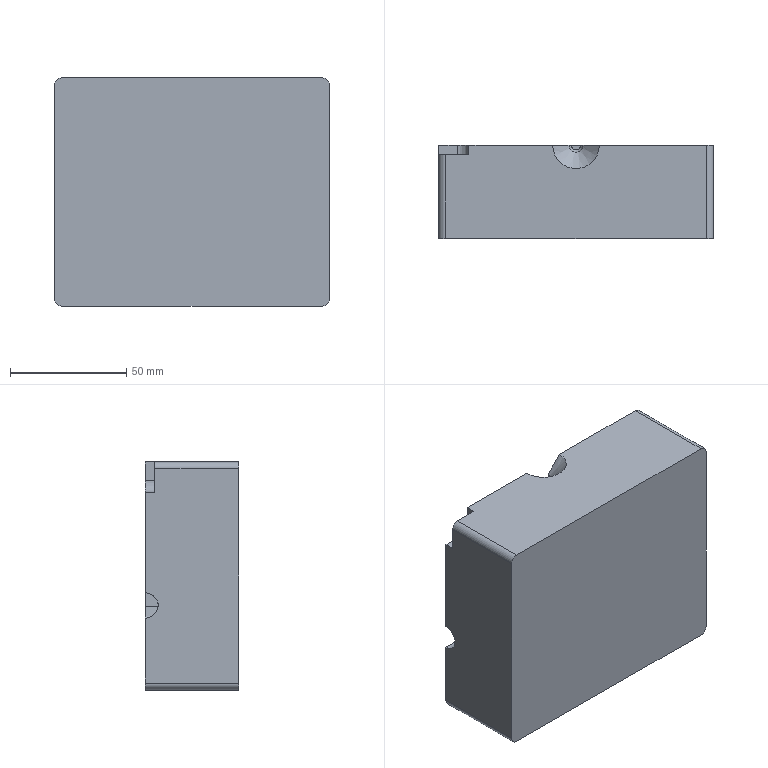NC program | NX | posted with a generic post | part box 118 x 40 x 98 mm
Lines 1488 to 2680 of 39656:
(CAVITY_MILL_COPY , TOOL : D4)
N2974 M6
N2976 G54
N2978 G17 G0 G90 X-30.742 Y-9.957 S0 M3
N2980 G43 Z30. H0
N2982 Z-0.963
N2984 G94 G1 Y-10.759 F250.
N2986 Y-17.85
N2988 X-31.058
N2990 Y-10.759
N2992 G2 X-33.146 Y-9.385 R2.52
N2994 X-33.058 Y-10.049 R2.146
N2996 G1 Y-19.85
N2998 X-28.742
N3000 Y-9.865
N3002 G2 X-28.696 Y-9.549 R1.086
N3004 G1 X-28.636 Y-9.352
N3006 X-28.053 Y-7.435
N3008 G0 X-33.789 Y-7.253 Z-1.925
N3010 G1 X-32.909 Y-9.083
N3012 X-32.861 Y-9.191
N3014 G2 X-32.701 Y-9.99 R2.527
N3016 G1 X-32.709 Y-10.
N3018 Y-19.814
N3020 G3 X-32.365 Y-19.85 R1.654
N3022 G1 X-29.435
N3024 X-29.112 Y-19.819
N3026 X-29.091 Y-19.815
N3028 Y-10.
N3030 X-29.098 Y-9.99
N3032 G2 X-28.879 Y-9.065 R2.165
N3034 G1 X-27.99 Y-7.245
N3036 G0 X-32.698 Y-7.471 Z-2.888
N3038 G1 X-33.034 Y-8.04
N3040 X-32.523 Y-8.656
N3042 X-32.418 Y-8.792
N3044 G2 X-32.042 Y-10. R2.079
N3046 G1 Y-19.671
N3048 G3 X-30.775 Y-19.785 R4.978
N3050 X-29.758 Y-19.671 R4.359
N3052 G1 Y-10.
N3054 G2 X-29.261 Y-8.64 R2.107
N3056 G1 X-28.745 Y-8.029
N3058 X-29.076 Y-7.457
N3060 G0 X-32.324 Y-7.137 Z-3.85
N3062 G1 X-32.463 Y-7.781
N3064 X-31.779 Y-8.197
N3066 G2 X-30.9 Y-9.216 R2.184
N3068 X-30.024 Y-8.196 R2.052
N3070 G1 X-29.333 Y-7.793
N3072 X-29.482 Y-7.134
N3074 G0 Z30.
N3076 X-34.354 Y-3.075
N3078 Z-0.963
N3080 G1 X-35.516 Y-4.812
N3082 G2 X-37.305 Y-5.764 R2.144
N3084 G1 X-37.919
N3086 Y-7.85
N3088 X-35.21
N3090 G2 X-34.483 Y-7.974 R2.146
N3092 G1 X-32.582 Y-8.651
N3094 G0 X-34.128 Y-2.971 Z-1.925
N3096 G1 X-35.263 Y-4.762
N3098 G2 X-37.084 Y-5.764 R2.157
N3100 G1 X-37.768
N3102 Y-7.85
N3104 X-34.875
N3106 G2 X-34.172 Y-7.965 R2.175
N3108 G1 X-32.249 Y-8.616
N3110 G0 X-33.73 Y-2.932 Z-2.888
N3112 G1 X-34.85 Y-4.742
N3114 G2 X-36.371 Y-5.734 R2.136
N3116 X-36.698 Y-5.764 R1.684
N3118 G1 X-37.51
N3120 Y-7.85
N3122 X-34.243
N3124 G2 X-33.618 Y-7.938 R2.232
N3126 G1 X-32.85 Y-8.161
N3128 X-32.462 Y-7.626
N3130 G0 X-33.123 Y-2.743 Z-3.85
N3132 G1 X-34.197 Y-4.658
N3134 G2 X-34.88 Y-5.395 R2.143
N3136 G1 X-35.172 Y-5.552
N3138 G2 X-36.111 Y-5.764 R2.188
N3140 G1 X-37.138
N3142 Y-7.85
N3144 X-33.069
N3146 G2 X-32.597 Y-7.898 R3.124
N3148 G1 X-31.81 Y-8.04
N3150 X-31.485 Y-7.443
N3152 G0 Z30.
N3154 X-58.08 Y13.101
N3156 Z-2.888
N3158 G1 X-57.261
N3160 X-40.113
N3162 G2 X-38.246 Y15.104 R2.52
N3164 G1 X-38.339 Y15.101
N3166 X-59.
N3168 X-61.015
N3170 X-39.295 Y12.219
N3172 X-40.113
N3174 X-57.261
N3176 G2 X-59. Y10.251 R2.52
N3178 G1 Y10.219
N3180 X-38.769
N3182 X-38.382 Y10.222
N3184 X-38.258 Y10.218
N3186 X-36.248 Y10.108
N3188 G0 Z30.
N3190 X-35.121 Y15.559
N3192 Z-3.85
N3194 G1 X-36.861 Y14.574
N3196 G2 X-37.896 Y14.301 R2.099
N3198 G1 X-58.975
N3200 X-59.
N3202 X-61.006 Y14.297
N3204 X-61. Y11.042
N3206 X-59. Y11.019
N3208 X-58.99
N3210 X-37.904
N3212 G2 X-36.839 Y10.731 R2.116
N3214 G1 X-35.105 Y9.72
N3216 G0 X-34.351 Y15.355 Z-4.814
N3218 G1 X-35.564 Y13.719
N3220 G2 X-37.25 Y12.869 R2.102
N3222 G1 X-37.57 Y12.871
N3224 X-58.975
N3226 X-59.
N3228 X-61.265 Y12.886
N3230 X-61.261 Y12.459
N3232 X-59. Y12.449
N3234 X-58.99
N3236 X-37.236
N3238 G2 X-35.971 Y12.02 R2.076
N3240 X-35.552 Y11.576 R2.175
N3242 G1 X-34.351 Y9.883
N3244 G0 Z30.
N3246 X-35.931 Y6.35
N3248 Z-0.963
N3250 G1 X-36.731
N3252 Y5.55
N3254 Y4.444
N3256 G2 X-36.041 Y4.113 R2.145
N3258 G1 X-34.406 Y2.929
N3260 G0 X-35.752 Y6.401 Z-1.925
N3262 G1 X-36.552
N3264 Y5.601
N3266 Y4.456
N3268 G2 X-35.793 Y4.096 R2.148
N3270 G1 X-34.173 Y2.89
N3272 G0 X-35.443 Y6.455 Z-2.888
N3274 G1 X-36.243
N3276 Y5.655
N3278 Y4.474
N3280 G2 X-35.504 Y4.17 R2.144
N3282 G1 X-33.813 Y3.068
N3284 G0 X-34.988 Y6.572 Z-3.85
N3286 G1 X-35.788
N3288 Y5.772
N3290 Y4.506
N3292 G2 X-34.943 Y4.188 R2.395
N3294 G1 X-33.225 Y3.136
N3296 G0 Z30.
N3298 X-34.351 Y6.757
N3300 Z-4.814
N3302 G1 X-35.151
N3304 Y5.957
N3306 Y4.564
N3308 G3 X-34.772 Y4.475 R4.427
N3310 G2 X-34.184 Y4.273 R2.191
N3312 G1 X-32.371 Y3.347
N3314 G0 Z30.
N3316 X-33.472 Y7.081
N3318 Z-5.778
N3320 G1 X-34.272
N3322 Y6.281
N3324 Y4.663
N3326 G3 X-33.573 Y4.51 R2.774
N3328 G2 X-32.997 Y4.395 R2.36
N3330 G1 X-32.237 Y4.143
N3332 X-31.834 Y4.675
N3334 G0 Z30.
N3336 X-27.389 Y2.955
N3338 Z-0.963
N3340 G1 X-25.745 Y4.124
N3342 G2 X-25.069 Y4.445 R2.143
N3344 G1 Y5.546
N3346 Y6.346
N3348 X-25.869
N3350 G0 X-27.61 Y2.981 Z-1.925
N3352 G1 X-25.953 Y4.135
N3354 G2 X-25.248 Y4.455 R2.149
N3356 G1 Y5.586
N3358 Y6.386
N3360 X-26.048
N3362 G0 X-27.99 Y3.049 Z-2.888
N3364 G1 X-26.303 Y4.163
N3366 G2 X-25.557 Y4.474 R2.153
N3368 G1 Y5.655
N3370 Y6.455
N3372 X-26.357
N3374 G0 X-28.58 Y3.121 Z-3.85
N3376 G1 X-26.843 Y4.198
N3378 G2 X-26.012 Y4.506 R2.239
N3380 G1 Y5.769
N3382 Y6.569
N3384 X-26.812
N3386 G0 X-29.417 Y3.37 Z-4.814
N3388 G1 X-27.611 Y4.277
N3390 G2 X-27.178 Y4.439 R2.146
N3392 G3 X-26.649 Y4.565 R3.444
N3394 G1 Y5.957
N3396 Y6.757
N3398 X-27.449
N3400 G0 Z30.
N3402 X-29.987 Y4.661
N3404 Z-5.778
N3406 G1 X-29.58 Y4.131
N3408 X-28.821 Y4.385
N3410 G2 X-28.295 Y4.497 R2.367
N3412 G3 X-27.528 Y4.663 R3.33
N3414 G1 Y6.281
N3416 Y7.081
N3418 X-28.328
N3420 G0 Z30.
N3422 X-22.377 Y13.101
N3424 Z-2.888
N3426 G1 X-21.092
N3428 X-19.388
N3430 G3 X-18.519 Y13.892 R2.
N3432 G2 X-16.717 Y15.101 R2.52
N3434 G1 X-23.426
N3436 X-23.549 Y15.105
N3438 X-25.552 Y15.217
N3440 G0 Z30.
N3442 X-18.179 Y12.219
N3444 Z-2.888
N3446 G1 X-19.541 Y12.22
N3448 X-20.998
N3450 G3 X-21.991 Y11.376 R2.
N3452 G2 X-23.535 Y10.219 R2.52
N3454 G1 X-23.417 Y10.222
N3456 X-23.181 Y10.219
N3458 X-17.313
N3460 G2 X-17.113 Y10.206 R2.13
N3462 G1 X-15.113 Y9.987
N3464 G0 Z30.
N3466 X-26.692 Y9.728
N3468 Z-3.85
N3470 G1 X-24.953 Y10.736
N3472 G2 X-24.083 Y11.014 R2.125
N3474 G1 X-23.913 Y11.021
N3476 X-23.581 Y11.019
N3478 X-17.287
N3480 G2 X-16.177 Y10.687 R2.053
N3482 G1 X-14.475 Y9.582
N3484 X-14.034 Y15.389
N3486 X-15.89 Y14.5
N3488 X-15.987 Y14.456
N3490 G2 X-16.798 Y14.301 R2.052
N3492 G1 X-23.581
N3494 X-23.892 Y14.297
N3496 G2 X-24.951 Y14.583 R2.119
N3498 G1 X-26.688 Y15.59
N3500 G0 X-27.449 Y9.952 Z-4.814
N3502 G1 X-26.24 Y11.594
N3504 G2 X-24.549 Y12.449 R2.1
N3506 G1 X-17.251
N3508 G2 X-15.587 Y11.58 R2.033
N3510 G1 X-15.522 Y11.481
N3512 X-14.351 Y9.618
N3514 X-13.97 Y15.475
N3516 X-15.424 Y13.642
N3518 G2 X-17.061 Y12.871 R2.039
N3520 G1 X-24.548
N3522 G2 X-26.242 Y13.729 R2.101
N3524 G1 X-27.449 Y15.375
N3526 G0 Z30.
N3528 X-15.428 Y-3.812
N3530 Z-0.963
N3532 G1 X-16.062 Y-3.445
N3534 X-16.573 Y-4.06
N3536 G2 X-20.207 Y-5.764 R4.725
N3538 G1 X-24.495
N3540 G2 X-26.289 Y-4.806 R2.143
N3542 G1 X-27.446 Y-3.062
N3544 X-29.223 Y-8.661
N3546 X-27.324 Y-7.977
N3548 G2 X-26.59 Y-7.85 R2.147
N3550 G1 X-14.726
N3552 X-13.926
N3554 Y-7.05
N3556 G0 X-15.428 Y-3.812 Z-1.925
N3558 G1 X-16.062 Y-3.445
N3560 X-16.573 Y-4.06
N3562 G2 X-20.207 Y-5.764 R4.725
N3564 G1 X-24.716
N3566 G2 X-26.528 Y-4.777 R2.157
N3568 G1 X-27.672 Y-3.004
N3570 X-29.536 Y-8.595
N3572 X-27.612 Y-7.959
N3574 G2 X-26.924 Y-7.85 R2.165
N3576 G1 X-14.726
N3578 X-13.926
N3580 Y-7.05
N3582 G0 X-15.428 Y-3.812 Z-2.888
N3584 G1 X-16.062 Y-3.445
N3586 X-16.573 Y-4.06
N3588 G2 X-20.207 Y-5.764 R4.725
N3590 G1 X-25.102
N3592 G2 X-26.952 Y-4.735 R2.154
N3594 G1 X-28.07 Y-2.912
N3596 X-29.351 Y-7.638
N3598 X-28.96 Y-8.17
N3600 X-28.193 Y-7.942
N3602 G2 X-27.557 Y-7.85 R2.228
N3604 G1 X-14.726
N3606 X-13.926
N3608 Y-7.05
N3610 G0 X-15.428 Y-3.812 Z-3.85
N3612 G1 X-16.062 Y-3.445
N3614 X-16.573 Y-4.06
N3616 G2 X-20.207 Y-5.764 R4.725
N3618 G1 X-25.689
N3620 G2 X-27.521 Y-4.795 R2.22
N3622 G1 X-27.594 Y-4.681
N3624 X-28.677 Y-2.845
N3626 X-30.266 Y-7.417
N3628 X-29.958 Y-8.021
N3630 X-29.169 Y-7.887
N3632 G2 X-28.73 Y-7.85 R2.566
N3634 G1 X-14.726
N3636 X-13.926
N3638 Y-7.05
N3640 G0 Z30.
N3642 X-30.794 Y2.521
N3644 Z-4.814
N3646 G1 Y1.72
N3648 Y-3.598
N3650 G3 X-30.138 Y-5.85 R4.087
N3652 G1 X-31.662
N3654 G3 X-31.006 Y-3.584 R4.091
N3656 G1 Y1.72
N3658 G2 X-33.098 Y3.001 R2.52
N3660 X-33.042 Y2.797 R2.191
N3662 G1 X-32.996 Y2.398
N3664 X-33.006 Y2.371
N3666 Y-3.597
N3668 G2 X-33.979 Y-5.395 R2.091
N3670 X-35.232 Y-5.764 R2.311
N3672 G1 X-36.63
N3674 Y-7.85
N3676 X-14.726
N3678 X-13.926
N3680 Y-7.05
N3682 X-15.428 Y-3.812
N3684 X-16.062 Y-3.445
N3686 X-16.573 Y-4.06
N3688 G2 X-20.207 Y-5.764 R4.725
N3690 G1 X-26.566
N3692 G2 X-27.239 Y-5.667 R2.948
N3694 X-27.578 Y-5.525 R1.364
N3696 X-28.794 Y-3.607 R2.087
N3698 G1 Y2.361
N3700 G2 X-28.68 Y3.05 R2.146
N3702 G1 X-28.028 Y4.969
N3704 G0 Z30.
N3706 X-15.428 Y-3.812
N3708 Z-5.778
N3710 G1 X-16.062 Y-3.445
N3712 X-16.573 Y-4.06
N3714 G2 X-20.207 Y-5.764 R4.725
N3716 G1 X-27.973
N3718 G2 X-29.592 Y-5.195 R2.509
N3720 X-30.322 Y-3.597 R2.013
N3722 G1 Y2.358
N3724 G2 X-29.605 Y3.939 R2.104
N3726 G1 X-29.004 Y4.467
N3728 X-29.25 Y5.079
N3730 X-32.538 Y5.078
N3732 X-32.792 Y4.46
N3734 X-32.19 Y3.934
N3736 G2 X-31.872 Y3.597 R2.36
N3738 X-31.478 Y2.35 R2.
N3740 G1 Y-3.628
N3742 G2 X-32.575 Y-5.452 R2.065
N3744 X-33.827 Y-5.764 R2.67
N3746 G1 X-35.963
N3748 Y-7.85
N3750 X-14.726
N3752 X-13.926
N3754 Y-7.05
N3756 G0 Z30.
N3758 X-30.802 Y50.223
N3760 Z-6.742
N3762 G1 Y48.36
N3764 Y6.616
N3766 X-30.998 Y6.617
N3768 Y48.36
N3770 G2 X-32.581 Y49. R2.52
N3772 G1 X-32.998
N3774 Y4.849
N3776 G3 X-32.374 Y4.705 R3.357
N3778 X-29.576 Y4.686 R12.401
N3780 X-28.802 Y4.848 R4.237
N3782 G1 Y49.
N3784 Y51.004
N3786 G0 Z30.
N3788 X-15.428 Y-3.812
N3790 Z-6.742
N3792 G1 X-16.062 Y-3.445
N3794 X-16.573 Y-4.06
N3796 G2 X-20.207 Y-5.764 R4.725
N3798 G1 X-35.086
N3800 Y-7.85
N3802 X-14.726
N3804 X-13.926
N3806 Y-7.05
N3808 G0 X-15.428 Y-3.812 Z-7.707
N3810 G1 X-16.062 Y-3.445
N3812 X-16.573 Y-4.06
N3814 G2 X-20.207 Y-5.764 R4.725
N3816 G1 X-33.596
N3818 X-33.894 Y-5.776
N3820 Y-7.85
N3822 X-14.726
N3824 X-13.926
N3826 Y-7.05
N3828 G0 X-15.422 Y-3.828 Z-8.671
N3830 G1 X-16.054 Y-3.458
N3832 X-16.568 Y-4.071
N3834 G2 X-19.94 Y-5.756 R4.731
N3836 X-20.207 Y-5.764 R4.725
N3838 G1 X-27.744
N3840 G3 X-30.975 Y-5.844 R72.062
N3842 X-32.076 Y-5.927 R18.052
N3844 G1 Y-7.832
N3846 X-31.974 Y-7.836
N3848 X-31.069 Y-7.85
N3850 X-14.714
N3852 X-13.914
N3854 Y-7.05
N3856 G0 X-14.831 Y-3.815 Z-9.635
N3858 G1 X-15.469 Y-3.48
N3860 X-15.973 Y-4.101
N3862 G2 X-17.236 Y-5.126 R3.966
N3864 X-19.883 Y-5.779 R5.896
N3866 G3 X-25.06 Y-5.994 R79.105
N3868 X-26.853 Y-6.206 R23.699
N3870 G1 Y-7.67
N3872 G3 X-24.38 Y-7.821 R33.331
N3874 G1 X-22.782 Y-7.849
N3876 X-22.62 Y-7.85
N3878 X-14.102
N3880 X-13.302
N3882 Y-7.05
N3884 G0 X-12.915 Y-2.639 Z-10.356
N3886 G1 X-14.194 Y-4.337
N3888 G2 X-14.486 Y-4.657 R2.325
N3890 X-17.42 Y-5.994 R5.27
N3892 G1 X-19.984 Y-6.253
N3894 X-20.157 Y-6.28
N3896 Y-7.613
N3898 G3 X-17.186 Y-7.789 R43.351
N3900 G1 X-16.387 Y-7.811
N3902 X-13.042 Y-7.85
N3904 X-12.204
N3906 X-11.404
N3908 Y-7.05
N3910 G0 Z30.
N3912 X-2.778 Y-8.134
N3914 Z-6.742
N3916 G1 X-2.373 Y-10.493
N3918 G2 X-2.385 Y-11.637 R3.183
N3920 G1 X-2.394 Y-11.678
N3922 X-2.546 Y-12.464
N3924 X-1.761 Y-12.616
N3926 G0 X-2.801 Y-8.096 Z-7.707
N3928 G1 X-2.364 Y-10.45
N3930 G2 X-2.368 Y-11.637 R3.183
N3932 G1 X-2.394 Y-11.767
N3934 X-2.546 Y-12.552
N3936 X-1.761 Y-12.705
N3938 G0 X-2.823 Y-8.052 Z-8.671
N3940 G1 X-2.35 Y-10.398
N3942 G2 X-2.346 Y-11.635 R3.178
N3944 G1 X-2.394 Y-11.881
N3946 X-2.546 Y-12.666
N3948 X-1.761 Y-12.818
N3950 G0 Z30.
N3952 X-0.177 Y-16.227
N3954 Z-9.635
N3956 G1 X-0.02 Y-15.418
N3958 X0. Y-15.318
N3960 X0.02 Y-15.418
N3962 G2 X2.394 Y-17.15 R2.52
N3964 G1 X1.313 Y-11.589
N3966 X1.244 Y-11.418
N3968 G2 X1.7 Y-9.701 R2.141
N3970 G1 X2.207 Y-9.082
N3972 X1.71 Y-8.538
N3974 X-1.733 Y-8.515
N3976 X-2.209 Y-9.052
N3978 X-1.706 Y-9.674
N3980 G2 X-1.23 Y-11.411 R2.247
N3982 G1 X-1.28 Y-11.423
N3984 X-2.394 Y-17.15
N3986 X-2.546 Y-17.936
N3988 X-1.761 Y-18.088
N3990 G0 Z30.
N3992 X-0.061 Y-7.471
N3994 Z-9.135
N3996 G3 X-0.061 Y-7.471 Z-9.185 I0.061 J0.456
N3998 X-0.061 Y-7.471 Z-9.236 I0.061 J0.456
N4000 X-0.061 Y-7.471 Z-9.286 I0.061 J0.456
N4002 X-0.061 Y-7.471 Z-9.337 I0.061 J0.456
N4004 X-0.061 Y-7.471 Z-9.387 I0.061 J0.456
N4006 X-0.061 Y-7.471 Z-9.438 I0.061 J0.456
N4008 X-0.061 Y-7.471 Z-9.488 I0.061 J0.456
N4010 X-0.061 Y-7.471 Z-9.539 I0.061 J0.456
N4012 X-0.061 Y-7.471 Z-9.589 I0.061 J0.456
N4014 X-0.061 Y-7.471 Z-9.639 I0.061 J0.456
N4016 X-0.061 Y-7.471 Z-9.69 I0.061 J0.456
N4018 X-0.061 Y-7.471 Z-9.74 I0.061 J0.456
N4020 X-0.061 Y-7.471 Z-9.791 I0.061 J0.456
N4022 X-0.061 Y-7.471 Z-9.841 I0.061 J0.456
N4024 X-0.061 Y-7.471 Z-9.892 I0.061 J0.456
N4026 X-0.061 Y-7.471 Z-9.942 I0.061 J0.456
N4028 X-0.061 Y-7.471 Z-9.993 I0.061 J0.456
N4030 X-0.061 Y-7.471 Z-10.043 I0.061 J0.456
N4032 X-0.061 Y-7.471 Z-10.094 I0.061 J0.456
N4034 X-0.061 Y-7.471 Z-10.144 I0.061 J0.456
N4036 X-0.061 Y-7.471 Z-10.194 I0.061 J0.456
N4038 X-0.061 Y-7.471 Z-10.245 I0.061 J0.456
N4040 X-0.061 Y-7.471 Z-10.295 I0.061 J0.456
N4042 X-0.061 Y-7.471 Z-10.346 I0.061 J0.456
N4044 X-0.061 Y-7.471 Z-10.396 I0.061 J0.456
N4046 X-0.061 Y-7.471 Z-10.447 I0.061 J0.456
N4048 X-0.061 Y-7.471 Z-10.497 I0.061 J0.456
N4050 X-0.061 Y-7.471 Z-10.548 I0.061 J0.456
N4052 X-0.061 Y-7.471 Z-10.598 I0.061 J0.456
N4054 X-0.061 Y-7.471 Z-10.648 I0.061 J0.456
N4056 X-0.061 Y-7.471 Z-10.699 I0.061 J0.456
N4058 X-0.061 Y-7.471 Z-10.749 I0.061 J0.456
N4060 X-0.061 Y-7.471 Z-10.8 I0.061 J0.456
N4062 X-0.061 Y-7.471 Z-10.85 I0.061 J0.456
N4064 X-0.061 Y-7.471 Z-10.901 I0.061 J0.456
N4066 X-0.061 Y-7.471 Z-10.951 I0.061 J0.456
N4068 X-0.061 Y-7.471 Z-11.002 I0.061 J0.456
N4070 X-0.061 Y-7.471 Z-11.052 I0.061 J0.456
N4072 X-0.061 Y-7.471 Z-11.103 I0.061 J0.456
N4074 X-0.061 Y-7.471 Z-11.153 I0.061 J0.456
N4076 X-0.061 Y-7.471 Z-11.203 I0.061 J0.456
N4078 X-0.061 Y-7.471 Z-11.254 I0.061 J0.456
N4080 X-0.061 Y-7.471 Z-11.304 I0.061 J0.456
N4082 X0. Y-7.475 Z-11.305 R0.46
N4084 X4.197 Y-7.406 R128.083
N4086 G1 Y-6.557
N4088 G3 X-4.197 Y-6.556 R87.806
N4090 G1 Y-7.407
N4092 G3 X0. Y-7.475 R128.083
N4094 G1 Y-6.675
N4096 G0 Z30.
N4098 X-3.997 Y-23.59
N4100 Z-0.963
N4102 G1 X-4.782 Y-23.437
N4104 X-4.935 Y-24.222
N4106 X-5.453 Y-26.888
N4108 X-2.737
N4110 X-1.937
N4112 Y-26.088
N4114 G0 X-3.976 Y-23.573 Z-1.925
N4116 G1 X-4.762 Y-23.42
N4118 X-4.914 Y-24.205
N4120 X-5.432 Y-26.871
N4122 X-2.717
N4124 X-1.917
N4126 Y-26.071
N4128 G0 X-3.956 Y-23.556 Z-2.888
N4130 G1 X-4.741 Y-23.403
N4132 X-4.894 Y-24.189
N4134 X-5.412 Y-26.855
N4136 X-2.696
N4138 X-1.896
N4140 Y-26.055
N4142 G0 X-3.936 Y-23.539 Z-3.85
N4144 G1 X-4.721 Y-23.387
N4146 X-4.874 Y-24.172
N4148 X-5.392 Y-26.838
N4150 X-2.676
N4152 X-1.876
N4154 Y-26.038
N4156 G0 X-3.915 Y-23.522 Z-4.814
N4158 G1 X-4.7 Y-23.37
N4160 X-4.853 Y-24.155
N4162 X-5.371 Y-26.821
N4164 X-2.655
N4166 X-1.855
N4168 Y-26.021
N4170 G0 X-3.895 Y-23.505 Z-5.778
N4172 G1 X-4.68 Y-23.353
N4174 X-4.833 Y-24.138
N4176 X-5.351 Y-26.804
N4178 X-2.635
N4180 X-1.835
N4182 Y-26.004
N4184 G0 X-3.874 Y-23.489 Z-6.742
N4186 G1 X-4.66 Y-23.336
N4188 X-4.812 Y-24.121
N4190 X-5.33 Y-26.787
N4192 X-2.615
N4194 X-1.815
N4196 Y-25.987
N4198 G0 X-3.854 Y-23.472 Z-7.707
N4200 G1 X-4.639 Y-23.319
N4202 X-4.792 Y-24.104
N4204 X-5.31 Y-26.77
N4206 X-2.594
N4208 X-1.794
N4210 Y-25.97
N4212 G0 X-3.828 Y-23.45 Z-8.671
N4214 G1 X-4.613 Y-23.297
N4216 X-4.765 Y-24.083
N4218 X-5.284 Y-26.749
N4220 X-2.568
N4222 X-1.768
N4224 Y-25.949
N4226 G0 Z30.
N4228 X-2.608 Y-22.445
N4230 Z-9.635
N4232 G1 X-3.393 Y-22.292
N4234 X-3.546 Y-23.077
N4236 X-4.064 Y-25.743
N4238 X-1.348
N4240 X-0.548
N4242 Y-24.943
N4244 G0 Z30.
N4246 X1.521 Y-44.826
N4248 Z-0.963
N4250 G1 X2.077 Y-44.248
N4252 X1.498 Y-43.696
N4254 G3 X1.353 Y-43.558 R155.055
N4256 G2 X0.683 Y-41.992 R2.116
N4258 G1 Y-32.
N4260 G3 X0.417 Y-31.459 R0.683
N4262 G2 X0. Y-31.036 R2.088
N4264 X-0.415 Y-31.458 R2.115
N4266 G3 X-0.683 Y-32. R0.683
N4268 G1 Y-42.
N4270 G2 X-1.353 Y-43.558 R2.118
N4272 G1 X-1.495 Y-43.693
N4274 X-2.074 Y-44.246
N4276 X-1.518 Y-44.823
N4278 G0 X1.118 Y-44.86 Z-1.925
N4280 G1 X1.632 Y-44.244
N4282 X1.322 Y-43.991
N4284 G3 X0.89 Y-43.644 R35.748
N4286 G2 X0.102 Y-42.015 R2.076
N4288 G1 Y-32.
N4290 G3 X0. Y-31.898 R0.102
N4292 X-0.102 Y-32. R0.102
N4294 G1 Y-42.019
N4296 G2 X-0.888 Y-43.642 R2.068
N4298 G3 X-1.32 Y-43.989 R35.652
N4300 G1 X-1.63 Y-44.242
N4302 X-1.116 Y-44.858
N4304 G0 X0.669 Y-45.191 Z-2.888
N4306 G1 X1.025 Y-44.473
N4308 G3 X0.4 Y-44.176 R5.552
N4310 X-0.4 Y-44.177 R1.105
N4312 X-1.024 Y-44.473 R5.541
N4314 G1 X-0.669 Y-45.191
N4316 G0 X0.281 Y-45.892 Z-3.85
N4318 G1 X0.428 Y-45.106
N4320 G3 X-0.428 Y-45.106 R2.16
N4322 G1 X-0.28 Y-45.893
N4324 G0 Z30.
N4326 X-2.74 Y-26.078
N4328 Z-0.963
N4330 G1 X-0.73 Y-27.138
N4332 G2 X0. Y-27.765 R2.163
N4334 X0.736 Y-27.134 R2.16
N4336 G1 X2.763 Y-26.074
N4338 G0 Z30.
N4340 X1.937 Y-26.088
N4342 Z-0.963
N4344 G1 Y-26.888
N4346 X2.737
N4348 X5.453
N4350 X4.935 Y-24.222
N4352 X4.782 Y-23.437
N4354 X3.997 Y-23.59
N4356 G0 X1.917 Y-26.071 Z-1.925
N4358 G1 Y-26.871
N4360 X2.717
N4362 X5.432
N4364 X4.914 Y-24.205
N4366 X4.762 Y-23.42
N4368 X3.976 Y-23.573
N4370 G0 X1.896 Y-26.055 Z-2.888
N4372 G1 Y-26.855
N4374 X2.696
N4376 X5.412
N4378 X4.894 Y-24.189
N4380 X4.741 Y-23.403
N4382 X3.956 Y-23.556
N4384 G0 X1.876 Y-26.038 Z-3.85
N4386 G1 Y-26.838
N4388 X2.676
N4390 X5.392
N4392 X4.874 Y-24.172
N4394 X4.721 Y-23.387
N4396 X3.936 Y-23.539
N4398 G0 X1.855 Y-26.021 Z-4.814
N4400 G1 Y-26.821
N4402 X2.655
N4404 X5.371
N4406 X4.853 Y-24.155
N4408 X4.7 Y-23.37
N4410 X3.915 Y-23.522
N4412 G0 X1.835 Y-26.004 Z-5.778
N4414 G1 Y-26.804
N4416 X2.635
N4418 X5.351
N4420 X4.833 Y-24.138
N4422 X4.68 Y-23.353
N4424 X3.895 Y-23.505
N4426 G0 X1.815 Y-25.987 Z-6.742
N4428 G1 Y-26.787
N4430 X2.615
N4432 X5.33
N4434 X4.812 Y-24.121
N4436 X4.66 Y-23.336
N4438 X3.874 Y-23.489
N4440 G0 X1.794 Y-25.97 Z-7.707
N4442 G1 Y-26.77
N4444 X2.594
N4446 X5.31
N4448 X4.792 Y-24.104
N4450 X4.639 Y-23.319
N4452 X3.854 Y-23.472
N4454 G0 X1.768 Y-25.949 Z-8.671
N4456 G1 Y-26.749
N4458 X2.568
N4460 X5.284
N4462 X4.765 Y-24.083
N4464 X4.613 Y-23.297
N4466 X3.828 Y-23.45
N4468 G0 Z30.
N4470 X0.548 Y-24.943
N4472 Z-9.635
N4474 G1 Y-25.743
N4476 X1.348
N4478 X4.064
N4480 X3.546 Y-23.077
N4482 X3.393 Y-22.292
N4484 X2.608 Y-22.445
N4486 G0 Z30.
N4488 X1.617 Y-11.876
N4490 Z-6.742
N4492 G1 X2.393 Y-11.675
N4494 G2 X2.372 Y-10.497 R3.182
N4496 G1 X2.775 Y-8.137
N4498 G0 X1.761 Y-12.705 Z-7.707
N4500 G1 X2.546 Y-12.552
N4502 X2.394 Y-11.767
N4504 X2.368 Y-11.637
N4506 G2 X2.362 Y-10.457 R3.18
N4508 G1 X2.794 Y-8.103
N4510 G0 X1.761 Y-12.818 Z-8.671
N4512 G1 X2.546 Y-12.666
N4514 X2.394 Y-11.881
N4516 X2.346 Y-11.635
N4518 G2 X2.348 Y-10.402 R3.163
N4520 G1 X2.816 Y-8.061
N4522 G0 Z30.
N4524 X27.446 Y-3.076
N4526 Z-0.963
N4528 G1 X26.286 Y-4.813
N4530 G2 X24.495 Y-5.764 R2.14
N4532 G1 X20.207
N4534 G2 X16.573 Y-4.06 R4.725
N4536 G1 X16.062 Y-3.445
N4538 X15.428 Y-3.812
N4540 X13.926 Y-7.05
N4542 Y-7.85
N4544 X14.726
N4546 X26.59
N4548 G2 X27.326 Y-7.979 R2.155
N4550 G1 X29.228 Y-8.666
N4552 G0 X27.672 Y-3.004 Z-1.925
N4554 G1 X26.528 Y-4.777
N4556 G2 X24.716 Y-5.764 R2.157
N4558 G1 X20.207
N4560 G2 X16.573 Y-4.06 R4.725
N4562 G1 X16.062 Y-3.445
N4564 X15.428 Y-3.812
N4566 X13.926 Y-7.05
N4568 Y-7.85
N4570 X14.726
N4572 X26.924
N4574 G2 X27.616 Y-7.961 R2.172
N4576 G1 X29.541 Y-8.602
N4578 G0 X28.07 Y-2.911 Z-2.888
N4580 G1 X26.952 Y-4.735
N4582 G2 X25.102 Y-5.764 R2.154
N4584 G1 X20.207
N4586 G2 X16.573 Y-4.06 R4.725
N4588 G1 X16.062 Y-3.445
N4590 X15.428 Y-3.812
N4592 X13.926 Y-7.05
N4594 Y-7.85
N4596 X14.726
N4598 X27.557
N4600 G2 X28.174 Y-7.933 R2.198
N4602 G1 X28.943 Y-8.151
N4604 X29.329 Y-7.617
N4606 G0 X28.677 Y-2.755 Z-3.85
N4608 G1 X27.602 Y-4.663
N4610 G2 X26.92 Y-5.395 R2.133
N4612 G1 X26.778 Y-5.473
N4614 G2 X25.689 Y-5.764 R2.208
N4616 G1 X20.207
N4618 G2 X16.573 Y-4.06 R4.725
N4620 G1 X16.062 Y-3.445
N4622 X15.428 Y-3.812
N4624 X13.926 Y-7.05
N4626 Y-7.85
N4628 X14.726
N4630 X28.73
N4632 G2 X29.155 Y-7.882 R2.453
N4634 G1 X29.945 Y-8.011
N4636 X30.254 Y-7.413
N4638 G0 Z30.
N4640 X25.869 Y6.354
N4642 Z-0.963
N4644 G1 X25.069
N4646 Y5.554
N4648 Y4.455
N4650 G2 X25.741 Y4.136 R2.147
N4652 G1 X27.388 Y2.968
N4654 G0 X26.048 Y6.395 Z-1.925
N4656 G1 X25.248
N4658 Y5.595
N4660 Y4.465
N4662 G2 X25.949 Y4.148 R2.144
N4664 G1 X27.608 Y2.999
N4666 G0 X26.357 Y6.469 Z-2.888
N4668 G1 X25.557
N4670 Y5.669
N4672 Y4.483
N4674 G2 X26.312 Y4.168 R2.148
N4676 G1 X27.993 Y3.05
N4678 G0 X26.812 Y6.583 Z-3.85
N4680 G1 X26.012
N4682 Y5.783
N4684 Y4.516
N4686 G2 X26.861 Y4.196 R2.289
N4688 G1 X28.584 Y3.117
N4690 G0 Z30.
N4692 X27.449 Y6.766
N4694 Z-4.814
N4696 G1 X26.649
N4698 Y5.966
N4700 Y4.575
N4702 X27.359 Y4.396
N4704 G2 X27.612 Y4.286 R2.228
N4706 G1 X29.433 Y3.356
N4708 G0 Z30.
N4710 X28.328 Y7.091
N4712 Z-5.778
N4714 G1 X27.528
N4716 Y6.291
N4718 Y4.675
N4720 G3 X28.377 Y4.501 R3.647
N4722 G2 X28.795 Y4.409 R2.266
N4724 G1 X29.557 Y4.165
N4726 X29.958 Y4.694
N4728 G0 Z30.
N4730 X34.411 Y2.965
N4732 Z-0.963
N4734 G1 X36.055 Y4.133
N4736 G2 X36.731 Y4.453 R2.143
N4738 G1 Y5.555
N4740 Y6.355
N4742 X35.931
N4744 G0 X34.171 Y2.886 Z-1.925
N4746 G1 X35.784 Y4.099
N4748 G2 X36.552 Y4.465 R2.146
N4750 G1 Y5.613
N4752 Y6.413
N4754 X35.752
N4756 G0 X33.808 Y3.065 Z-2.888
N4758 G1 X35.5 Y4.176
N4760 G2 X36.243 Y4.485 R2.16
N4762 G1 Y5.666
N4764 Y6.466
N4766 X35.443
N4768 G0 X33.227 Y3.153 Z-3.85
N4770 G1 X34.946 Y4.202
N4772 G2 X35.172 Y4.322 R2.133
N4774 X35.788 Y4.518 R2.795
N4776 G1 Y5.783
N4778 Y6.583
N4780 X34.988
N4782 G0 X32.39 Y3.391 Z-4.814
N4784 G1 X34.201 Y4.293
N4786 G2 X34.772 Y4.483 R2.155
N4788 G3 X35.151 Y4.575 R2.012
N4790 G1 Y5.963
N4792 Y6.763
N4794 X34.351
N4796 G0 Z30.
N4798 X31.801 Y4.671
N4800 Z-5.778
N4802 G1 X32.213 Y4.136
N4804 X32.972 Y4.391
N4806 G2 X33.573 Y4.519 R2.714
N4808 G3 X34.272 Y4.676 R2.469
N4810 G1 Y6.29
N4812 Y7.09
N4814 X33.472
N4816 G0 Z30.
N4818 X32.582 Y-8.65
N4820 Z-0.963
N4822 G1 X34.484 Y-7.974
N4824 G2 X35.21 Y-7.85 R2.145
N4826 G1 X37.919
N4828 Y-5.764
N4830 X37.305
N4832 G2 X35.521 Y-4.819 R2.145
N4834 G1 X34.354 Y-3.091
N4836 G0 X32.251 Y-8.618 Z-1.925
N4838 G1 X34.17 Y-7.966
N4840 G2 X34.875 Y-7.85 R2.186
N4842 G1 X37.768
N4844 Y-5.764
N4846 X37.084
N4848 G2 X35.261 Y-4.758 R2.157
N4850 G1 X34.128 Y-2.963
N4852 G0 X32.458 Y-7.628 Z-2.888
N4854 G1 X32.846 Y-8.169
N4856 X33.613 Y-7.942
N4858 G2 X34.243 Y-7.85 R2.225
N4860 G1 X37.51
N4862 Y-5.764
N4864 X36.698
N4866 G2 X35.479 Y-5.395 R2.273
N4868 X34.857 Y-4.756 R2.135
N4870 G1 X33.73 Y-2.961
N4872 G0 X31.509 Y-7.43 Z-3.85
N4874 G1 X31.829 Y-8.031
N4876 X32.617 Y-7.894
N4878 G2 X33.069 Y-7.85 R3.034
N4880 G1 X37.138
N4882 Y-5.764
N4884 X36.111
N4886 G2 X34.204 Y-4.671 R2.193
N4888 G1 X33.123 Y-2.807
N4890 G0 Z30.
N4892 X31.006 Y2.531
N4894 Z-4.814
N4896 G1 Y1.73
N4898 Y-3.571
N4900 G3 X31.487 Y-5.551 R3.968
N4902 X31.666 Y-5.85 R4.24
N4904 G1 X30.138
N4906 G3 X30.794 Y-3.598 R4.093
N4908 G1 Y1.729
N4910 G2 X28.704 Y3.008 R2.52
N4912 X28.794 Y2.372 R2.224
N4914 G1 Y-3.607
N4916 G2 X28.088 Y-5.195 R2.093
N4918 X26.566 Y-5.764 R2.33
N4920 G1 X20.207
N4922 G2 X16.573 Y-4.06 R4.725
N4924 G1 X16.062 Y-3.445
N4926 X15.428 Y-3.812
N4928 X13.926 Y-7.05
N4930 Y-7.85
N4932 X14.726
N4934 X36.63
N4936 Y-5.764
N4938 X35.232
N4940 G2 X33.244 Y-4.596 R2.24
N4942 X33.006 Y-3.597 R1.968
N4944 G1 Y2.36
N4946 G2 X33.124 Y3.066 R2.155
N4948 G1 X33.786 Y4.988
N4950 G0 X29.269 Y5.088 Z-5.778
N4952 G1 X29.017 Y4.474
N4954 X29.613 Y3.941
N4956 G2 X30.162 Y3.2 R2.266
N4958 X30.322 Y2.472 R1.739
N4960 G1 Y-3.636
N4962 G2 X29.176 Y-5.469 R2.04
N4964 X27.973 Y-5.764 R2.448
N4966 G1 X20.207
N4968 G2 X16.573 Y-4.06 R4.725
N4970 G1 X16.062 Y-3.445
N4972 X15.428 Y-3.812
N4974 X13.926 Y-7.05
N4976 Y-7.85
N4978 X14.726
N4980 X35.963
N4982 Y-5.764
N4984 X33.827
N4986 G2 X32.575 Y-5.452 R2.67
N4988 X31.478 Y-3.628 R2.065
N4990 G1 Y2.36
N4992 G2 X32.15 Y3.92 R2.077
N4994 G1 X32.739 Y4.461
N4996 X32.489 Y5.063
N4998 G0 Z30.
N5000 X13.926 Y-7.05
N5002 Z-6.742
N5004 G1 Y-7.85
N5006 X14.726
N5008 X35.086
N5010 Y-5.764
N5012 X20.207
N5014 G2 X16.573 Y-4.06 R4.725
N5016 G1 X16.062 Y-3.445
N5018 X15.428 Y-3.812
N5020 G0 X13.926 Y-7.05 Z-7.707
N5022 G1 Y-7.85
N5024 X14.726
N5026 X33.894
N5028 Y-5.775
N5030 X33.594 Y-5.764
N5032 X20.207
N5034 G2 X16.573 Y-4.06 R4.725
N5036 G1 X16.062 Y-3.445
N5038 X15.428 Y-3.812
N5040 G0 X13.911 Y-7.05 Z-8.671
N5042 G1 Y-7.85
N5044 X14.711
N5046 X31.07
N5048 X31.974 Y-7.836
N5050 X32.076 Y-7.832
N5052 Y-5.926
N5054 G3 X30.7 Y-5.832 R28.182
N5056 X27.744 Y-5.764 R71.547
N5058 G1 X20.207
N5060 G2 X19.983 Y-5.759 R4.725
N5062 X16.555 Y-4.054 R4.733
N5064 G1 X16.044 Y-3.438
N5066 X15.41 Y-3.806
N5068 G0 X13.301 Y-7.05 Z-9.635
N5070 G1 Y-7.85
N5072 X14.101
N5074 X22.62
N5076 G3 X25.18 Y-7.791 R75.43
N5078 X26.853 Y-7.671 R30.215
N5080 G1 Y-6.206
N5082 G3 X24.044 Y-5.921 R32.027
N5084 X19.796 Y-5.778 R91.855
N5086 G2 X17.186 Y-5.1 R5.823
N5088 X15.957 Y-4.074 R3.998
N5090 G1 X15.458 Y-3.448
N5092 X14.817 Y-3.779
N5094 G0 Z30.
N5096 X11.39 Y-7.05
N5098 Z-10.356
N5100 G1 Y-7.85
N5102 X12.19
N5104 X13.036
N5106 X16.387 Y-7.811
N5108 X17.186 Y-7.789
N5110 G3 X20.157 Y-7.613 R42.858
N5112 G1 Y-6.28
N5114 G3 X17.461 Y-5.994 R142.428
N5116 G2 X14.388 Y-4.547 R5.023
N5118 X14.144 Y-4.259 R2.252
N5120 G1 X12.912 Y-2.529
N5122 G0 Z30.
N5124 X30.998 Y50.23
N5126 Z-6.742
N5128 G1 Y48.363
N5130 Y6.627
N5132 X30.802
N5134 Y48.363
N5136 G2 X29.222 Y49. R2.52
N5138 G1 X28.802
N5140 Y48.991
N5142 Y4.858
N5144 G3 X29.576 Y4.695 R4.283
N5146 X32.066 Y4.68 R12.927
N5148 X32.998 Y4.856 R4.909
N5150 G1 Y48.976
N5152 X32.997 Y49.
N5154 X32.981 Y51.
N5156 G0 Z30.
N5158 X31.058 Y-9.959
N5160 Z-0.963
N5162 G1 Y-10.762
N5164 Y-17.85
N5166 X30.742
N5168 Y-10.762
N5170 G2 X28.664 Y-9.41 R2.52
N5172 G1 X28.708 Y-9.591
N5174 G2 X28.742 Y-9.945 R1.842
N5176 G1 Y-19.85
N5178 X33.058
N5180 Y-10.002
N5182 G2 X33.144 Y-9.394 R2.145
N5184 G1 X33.709 Y-7.457
N5186 G0 X27.991 Y-7.246 Z-1.925
N5188 G1 X28.881 Y-9.068
N5190 G2 X29.062 Y-9.61 R2.172
N5192 X29.093 Y-9.942 R1.71
N5194 G1 X29.091 Y-10.39
N5196 Y-19.812
N5198 X29.107 Y-19.816
N5200 X29.435 Y-19.85
N5202 X32.365
N5204 X32.684 Y-19.82
N5206 X32.709 Y-19.815
N5208 Y-10.
N5210 X32.701 Y-9.99
N5212 G2 X32.92 Y-9.068 R2.198
N5214 G1 X33.798 Y-7.25
N5216 G0 X29.09 Y-7.461 Z-2.888
N5218 G1 X28.757 Y-8.029
N5220 X29.267 Y-8.645
N5222 G2 X29.672 Y-9.391 R2.198
N5224 X29.758 Y-9.949 R1.868
N5226 G1 Y-19.672
N5228 G3 X30.775 Y-19.785 R4.013
N5230 X32.042 Y-19.671 R4.773
N5232 G1 Y-9.995
N5234 G2 X32.529 Y-8.647 R2.11
N5236 G1 X33.04 Y-8.031
N5238 X32.718 Y-7.463
N5240 G0 X29.47 Y-7.128 Z-3.85
N5242 G1 X29.323 Y-7.785
N5244 X30.011 Y-8.193
N5246 G2 X30.518 Y-8.592 R2.453
N5248 X30.899 Y-9.216 R2.173
N5250 X31.785 Y-8.193 R2.185
N5252 G1 X32.471 Y-7.78
N5254 X32.332 Y-7.135
N5256 G0 Z30.
N5258 M5
(FACE_MILLING , TOOL : D8)
N5260 M6
N5262 G54
N5264 G17 G0 G90 X-50.9 Y39. S0 M3
N5266 G43 Z30. H0
N5268 Z-16.5
N5270 G94 G1 Z-20. F250.
N5272 G3 X-49. Y37.1 R1.9
N5274 X-50.9 Y39. R-1.9
N5276 G1 X-48.9
N5278 G0 Z30.
N5280 X-56. Y-57.
N5282 Z-4.
N5284 G1 Y-49.
N5286 Y-46.
N5288 X-59.
N5290 X-67.
N5292 X-50. Y-57.
N5294 Y-49.
N5296 Y-41.
N5298 G3 X-51. Y-40. R1.
N5300 G1 X-59.
N5302 X-67.
N5304 G0 Z30.
N5306 X49. Y-40.9
N5308 Z-16.5
N5310 G1 Z-20.
N5312 G3 X50.9 Y-39. R1.9
N5314 X49. Y-40.9 R-1.9
N5316 G1 Y-38.9
N5318 G0 Z30.
N5320 X56. Y57.
N5322 Z-4.
N5324 G1 Y49.
N5326 Y46.
N5328 X59.
N5330 X67.
N5332 X50. Y57.
N5334 Y49.
N5336 Y41.
N5338 G3 X51. Y40. R1.
N5340 G1 X59.
N5342 X67.
N5344 G0 Z30.
N5346 M5